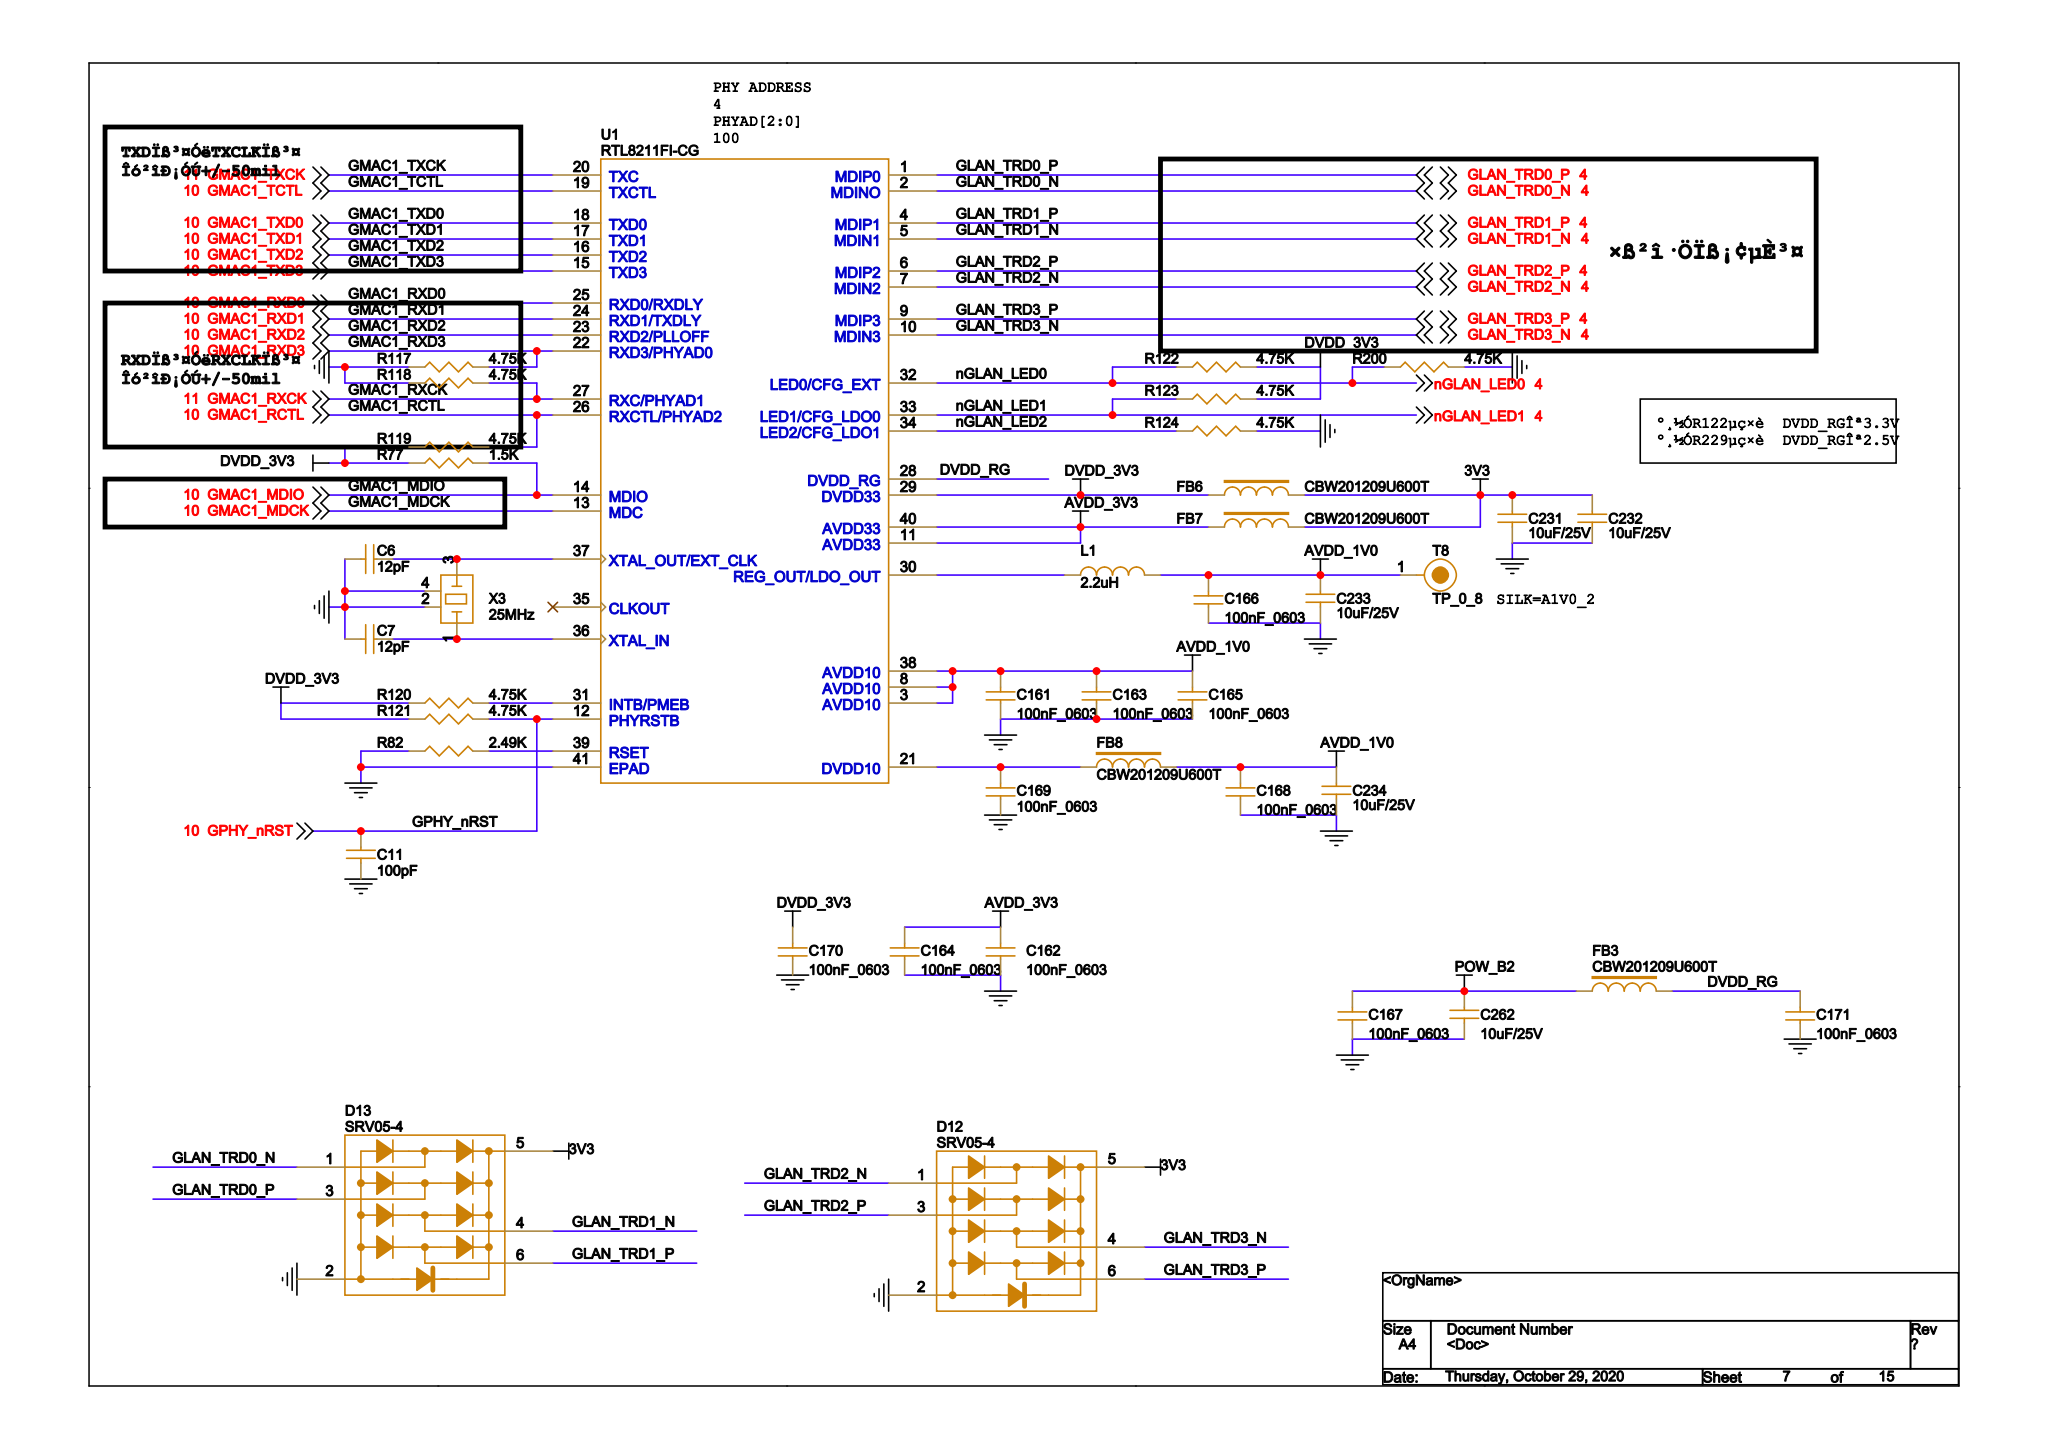Circuit board | Cadence Allegro | 406 parts | 392 nets | one sheet of the schematic
Parts on this sheet (reference | value | footprint):
C6 | 12pF | C_0603
C7 | 12pF | C_0603
C11 | 100pF | C_0603
C161 | 100nF_0603 | C_0603_104
C162 | 100nF_0603 | C_0603_104
C163 | 100nF_0603 | C_0603_104
C164 | 100nF_0603 | C_0603_104
C165 | 100nF_0603 | C_0603_104
C166 | 100nF_0603 | C_0603_104
C167 | 100nF_0603 | C_0603_104
C168 | 100nF_0603 | C_0603_104
C169 | 100nF_0603 | C_0603_104
C170 | 100nF_0603 | C_0603_104
C171 | 100nF_0603 | C_0603_104
C231 | 10uF/25V | C_0805_106
C232 | 10uF/25V | C_0805_106
C233 | 10uF/25V | C_0805_106
C234 | 10uF/25V | C_0805_106
C262 | 10uF/25V | C_0805_106
D12 | SRV05-4 | D_SOT23_6
D13 | SRV05-4 | D_SOT23_6
FB3 | CBW201209U600T | L_0805
FB6 | CBW201209U600T | L_0805
FB7 | CBW201209U600T | L_0805
FB8 | CBW201209U600T | L_0805
L1 | 2.2uH | L_SDB0530
R77 | 1.5K | R_0603
R82 | 2.49K | R_0603
R117 | 4.75K | R_0603
R118 | 4.75K | R_0603
R119 | 4.75K | R_0603
R120 | 4.75K | R_0603
R121 | 4.75K | R_0603
R122 | 4.75K | R_0603
R123 | 4.75K | R_0603
R124 | 4.75K | R_0603
R200 | 4.75K | R_0603
T8 | TP_0_8 | TP_0_8
U1 | RTL8211FI-CG | U_QFN40_0_4
X3 | 25MHz | XTAL3225
Nets of these parts (net: part-pin ...):
GND: C6-2 C7-2 C11-2 C161-1 C162-1 C163-1 C164-1 C165-1 C166-1 C167-1 C168-1 C169-1 C170-1 C171-1 C231-2 C232-2 C233-2 C234-2 C262-2 D12-2 D13-2 R82-1 R117-1 R118-1 R124-2 R200-2 X3-2 X3-4 U1-41
GLAN_TRD0_P: D13-3 U1-1
GLAN_TRD0_N: D13-1 U1-2
GLAN_TRD1_P: D13-6 U1-4
GLAN_TRD1_N: D13-4 U1-5
GLAN_TRD2_P: D12-3 U1-6
GLAN_TRD2_N: D12-1 U1-7
GLAN_TRD3_P: D12-6 U1-9
GLAN_TRD3_N: D12-4 U1-10
NGLAN_LED0: R122-1 R200-1 U1-32
NGLAN_LED1: R123-1 U1-33
POW_B2: C167-2 C262-1 FB3-1
3V3: C231-1 C232-1 D12-5 D13-5 FB6-2 FB7-2
GPHY_NRST: C11-1 R121-2 U1-12
AVDD_1V0: C161-2 C163-2 C165-2 C166-2 C168-2 C233-1 C234-1 FB8-2 L1-2 T8-1 U1-3 U1-8 U1-38
AVDD_3V3: C162-2 C164-2 FB7-1 U1-11 U1-40
N20019298: C169-2 FB8-1 U1-21
DVDD_3V3: C170-2 FB6-1 R77-1 R119-1 R120-1 R121-1 R122-2 R123-2 U1-29
DVDD_RG: C171-2 FB3-2 U1-28
N20019192: C6-1 X3-3 U1-37
N20019204: C7-1 X3-1 U1-36
N20019284: L1-1 U1-30
GMAC1_RXD3: R117-2 U1-22
GMAC1_RXCK: R118-2 U1-27
GMAC1_RCTL: R119-2 U1-26
N20019252: R120-2 U1-31
NGLAN_LED2: R124-1 U1-34
GMAC1_MDIO: R77-2 U1-14
N20019154: R82-2 U1-39
GMAC1_MDCK: U1-13
GMAC1_RXD0: U1-25
GMAC1_RXD1: U1-24
GMAC1_RXD2: U1-23
GMAC1_TXCK: U1-20
GMAC1_TCTL: U1-19
GMAC1_TXD0: U1-18
GMAC1_TXD1: U1-17
GMAC1_TXD2: U1-16
GMAC1_TXD3: U1-15